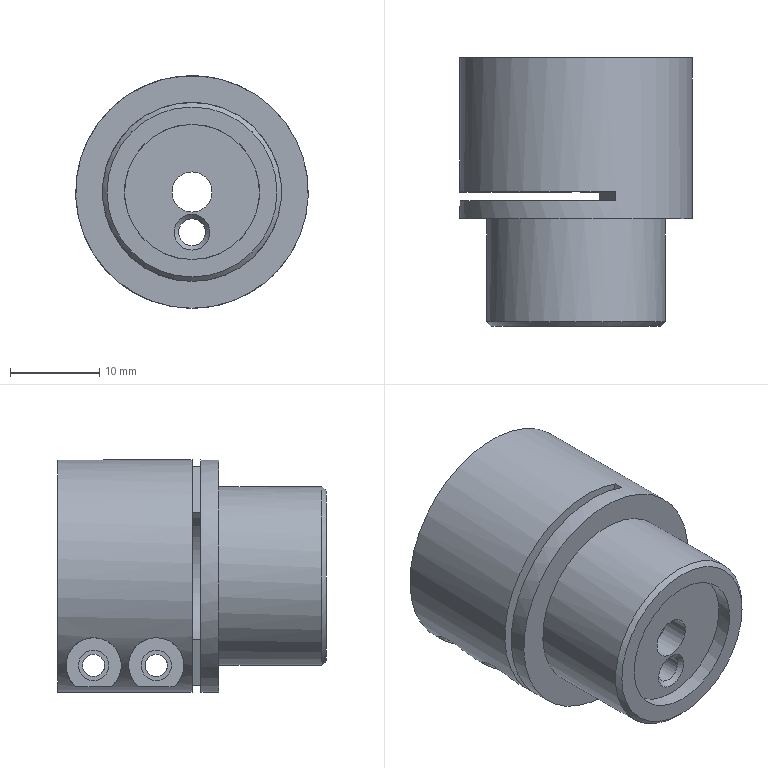Part | NX | 1 solid | 33 faces | box 26 x 30 x 26 mm | volume 7708 mm3 | plane 17 | cylinder 13 | cone 3 | commonest cylinder face diameters 15.1 x3 2.5 x2 3.4 x2 6.2 x2 3 x1 4.5 x1
STEP:
#1=CARTESIAN_POINT('',(0.,-15.,9.5));
#2=VERTEX_POINT('',#1);
#3=CARTESIAN_POINT('',(0.,-15.,0.));
#4=DIRECTION('',(0.,1.,0.));
#5=DIRECTION('',(0.,0.,1.));
#6=AXIS2_PLACEMENT_3D('',#3,#4,#5);
#7=CIRCLE('',#6,9.5);
#8=EDGE_CURVE('',#2,#2,#7,.F.);
#9=ORIENTED_EDGE('',*,*,#8,.T.);
#10=EDGE_LOOP('',(#9));
#11=FACE_BOUND('',#10,.T.);
#12=CARTESIAN_POINT('',(0.,-15.,7.55));
#13=VERTEX_POINT('',#12);
#14=CARTESIAN_POINT('',(0.,-15.,0.));
#15=DIRECTION('',(0.,1.,0.));
#16=DIRECTION('',(0.,0.,1.));
#17=AXIS2_PLACEMENT_3D('',#14,#15,#16);
#18=CIRCLE('',#17,7.55);
#19=EDGE_CURVE('',#13,#13,#18,.T.);
#20=ORIENTED_EDGE('',*,*,#19,.T.);
#21=EDGE_LOOP('',(#20));
#22=FACE_BOUND('',#21,.T.);
#23=CARTESIAN_POINT('',(0.,-15.,0.));
#24=DIRECTION('',(0.,1.,0.));
#25=DIRECTION('',(0.,0.,1.));
#26=AXIS2_PLACEMENT_3D('',#23,#24,#25);
#27=PLANE('',#26);
#28=ADVANCED_FACE('',(#11,#22),#27,.F.);
#29=CARTESIAN_POINT('',(4.446,-1.,12.216));
#30=VERTEX_POINT('',#29);
#31=CARTESIAN_POINT('',(4.446,0.,12.216));
#32=VERTEX_POINT('',#31);
#33=CARTESIAN_POINT('',(4.446,15.,12.216));
#34=DIRECTION('',(0.,-1.,0.));
#35=VECTOR('',#34,1000.);
#36=LINE('',#33,#35);
#37=EDGE_CURVE('',#30,#32,#36,.F.);
#38=ORIENTED_EDGE('',*,*,#37,.F.);
#39=CARTESIAN_POINT('',(4.446,-1.,-12.216));
#40=VERTEX_POINT('',#39);
#41=CARTESIAN_POINT('',(0.,-1.,0.));
#42=DIRECTION('',(0.,1.,0.));
#43=DIRECTION('',(0.,0.,1.));
#44=AXIS2_PLACEMENT_3D('',#41,#42,#43);
#45=CIRCLE('',#44,13.);
#46=EDGE_CURVE('',#40,#30,#45,.T.);
#47=ORIENTED_EDGE('',*,*,#46,.F.);
#48=CARTESIAN_POINT('',(4.446,0.,-12.216));
#49=VERTEX_POINT('',#48);
#50=CARTESIAN_POINT('',(4.446,15.,-12.216));
#51=DIRECTION('',(0.,-1.,0.));
#52=VECTOR('',#51,1000.);
#53=LINE('',#50,#52);
#54=EDGE_CURVE('',#40,#49,#53,.F.);
#55=ORIENTED_EDGE('',*,*,#54,.T.);
#56=CARTESIAN_POINT('',(0.5,0.,-12.99));
#57=VERTEX_POINT('',#56);
#58=CARTESIAN_POINT('',(0.,0.,0.));
#59=DIRECTION('',(0.,1.,0.));
#60=DIRECTION('',(0.,0.,1.));
#61=AXIS2_PLACEMENT_3D('',#58,#59,#60);
#62=CIRCLE('',#61,13.);
#63=EDGE_CURVE('',#49,#57,#62,.T.);
#64=ORIENTED_EDGE('',*,*,#63,.T.);
#65=CARTESIAN_POINT('',(0.5,15.,-12.99));
#66=VERTEX_POINT('',#65);
#67=CARTESIAN_POINT('',(0.5,15.,-12.99));
#68=DIRECTION('',(0.,-1.,0.));
#69=VECTOR('',#68,1000.);
#70=LINE('',#67,#69);
#71=EDGE_CURVE('',#57,#66,#70,.F.);
#72=ORIENTED_EDGE('',*,*,#71,.T.);
#73=CARTESIAN_POINT('',(-0.5,15.,-12.99));
#74=VERTEX_POINT('',#73);
#75=CARTESIAN_POINT('',(0.,15.,0.));
#76=DIRECTION('',(0.,1.,0.));
#77=DIRECTION('',(0.,0.,1.));
#78=AXIS2_PLACEMENT_3D('',#75,#76,#77);
#79=CIRCLE('',#78,13.);
#80=EDGE_CURVE('',#74,#66,#79,.T.);
#81=ORIENTED_EDGE('',*,*,#80,.F.);
#82=CARTESIAN_POINT('',(-0.5,0.,-12.99));
#83=VERTEX_POINT('',#82);
#84=CARTESIAN_POINT('',(-0.5,15.,-12.99));
#85=DIRECTION('',(0.,-1.,0.));
#86=VECTOR('',#85,1000.);
#87=LINE('',#84,#86);
#88=EDGE_CURVE('',#74,#83,#87,.T.);
#89=ORIENTED_EDGE('',*,*,#88,.T.);
#90=CARTESIAN_POINT('',(0.,0.,0.));
#91=DIRECTION('',(0.,1.,0.));
#92=DIRECTION('',(0.,0.,1.));
#93=AXIS2_PLACEMENT_3D('',#90,#91,#92);
#94=CIRCLE('',#93,13.);
#95=EDGE_CURVE('',#83,#32,#94,.T.);
#96=ORIENTED_EDGE('',*,*,#95,.T.);
#97=EDGE_LOOP('',(#38,#47,#55,#64,#72,#81,#89,#96));
#98=FACE_BOUND('',#97,.T.);
#99=CARTESIAN_POINT('',(-4.,5.999,-12.369));
#100=VERTEX_POINT('',#99);
#101=CARTESIAN_POINT('',(-4.,2.001,-12.369));
#102=VERTEX_POINT('',#101);
#103=CARTESIAN_POINT('',(-4.,5.999,-12.369));
#104=CARTESIAN_POINT('',(-4.809,6.309,-12.108));
#105=CARTESIAN_POINT('',(-6.367,6.865,-11.433));
#106=CARTESIAN_POINT('',(-8.603,7.27,-9.884));
#107=CARTESIAN_POINT('',(-10.159,6.725,-8.173));
#108=CARTESIAN_POINT('',(-10.887,5.376,-7.115));
#109=CARTESIAN_POINT('',(-11.081,4.013,-6.796));
#110=CARTESIAN_POINT('',(-10.895,2.65,-7.102));
#111=CARTESIAN_POINT('',(-10.168,1.277,-8.163));
#112=CARTESIAN_POINT('',(-8.611,0.7311,-9.877));
#113=CARTESIAN_POINT('',(-6.379,1.131,-11.427));
#114=CARTESIAN_POINT('',(-4.811,1.69,-12.107));
#115=CARTESIAN_POINT('',(-4.,2.001,-12.369));
#116=B_SPLINE_CURVE_WITH_KNOTS('',3,(#103,#104,#105,#106,#107,#108,#109,#110,#111,#112,#113,#114,#115),.UNSPECIFIED.,.F.,.F.,(4,1,1,1,1,1,1,1,1,1,4),(0.,0.00268,0.00536,0.008039,0.009379,0.01072,0.01206,0.0134,0.01608,0.01876,0.02144),.UNSPECIFIED.);
#117=EDGE_CURVE('',#100,#102,#116,.T.);
#118=ORIENTED_EDGE('',*,*,#117,.T.);
#119=CARTESIAN_POINT('',(-4.,15.,-12.369));
#120=DIRECTION('',(0.,-1.,0.));
#121=VECTOR('',#120,1000.);
#122=LINE('',#119,#121);
#123=EDGE_CURVE('',#102,#100,#122,.F.);
#124=ORIENTED_EDGE('',*,*,#123,.T.);
#125=EDGE_LOOP('',(#118,#124));
#126=FACE_BOUND('',#125,.T.);
#127=CARTESIAN_POINT('',(-4.,12.999,-12.369));
#128=VERTEX_POINT('',#127);
#129=CARTESIAN_POINT('',(-4.,9.001,-12.369));
#130=VERTEX_POINT('',#129);
#131=CARTESIAN_POINT('',(-4.,12.999,-12.369));
#132=CARTESIAN_POINT('',(-4.809,13.309,-12.108));
#133=CARTESIAN_POINT('',(-6.367,13.865,-11.433));
#134=CARTESIAN_POINT('',(-8.603,14.27,-9.884));
#135=CARTESIAN_POINT('',(-10.159,13.725,-8.173));
#136=CARTESIAN_POINT('',(-10.887,12.376,-7.115));
#137=CARTESIAN_POINT('',(-11.081,11.013,-6.796));
#138=CARTESIAN_POINT('',(-10.895,9.65,-7.102));
#139=CARTESIAN_POINT('',(-10.168,8.277,-8.163));
#140=CARTESIAN_POINT('',(-8.611,7.731,-9.877));
#141=CARTESIAN_POINT('',(-6.379,8.131,-11.427));
#142=CARTESIAN_POINT('',(-4.811,8.69,-12.107));
#143=CARTESIAN_POINT('',(-4.,9.001,-12.369));
#144=B_SPLINE_CURVE_WITH_KNOTS('',3,(#131,#132,#133,#134,#135,#136,#137,#138,#139,#140,#141,#142,#143),.UNSPECIFIED.,.F.,.F.,(4,1,1,1,1,1,1,1,1,1,4),(0.,0.00268,0.00536,0.008039,0.009379,0.01072,0.01206,0.0134,0.01608,0.01876,0.02144),.UNSPECIFIED.);
#145=EDGE_CURVE('',#128,#130,#144,.T.);
#146=ORIENTED_EDGE('',*,*,#145,.T.);
#147=CARTESIAN_POINT('',(-4.,15.,-12.369));
#148=DIRECTION('',(0.,-1.,0.));
#149=VECTOR('',#148,1000.);
#150=LINE('',#147,#149);
#151=EDGE_CURVE('',#130,#128,#150,.F.);
#152=ORIENTED_EDGE('',*,*,#151,.T.);
#153=EDGE_LOOP('',(#146,#152));
#154=FACE_BOUND('',#153,.T.);
#155=CARTESIAN_POINT('',(9.614,4.,-8.75));
#156=VERTEX_POINT('',#155);
#157=CARTESIAN_POINT('',(9.506,3.358,-8.871));
#158=CARTESIAN_POINT('',(9.669,4.,-8.69));
#159=CARTESIAN_POINT('',(9.506,4.642,-8.871));
#160=CARTESIAN_POINT('',(9.013,5.175,-9.383));
#161=CARTESIAN_POINT('',(8.2,5.33,-10.117));
#162=CARTESIAN_POINT('',(7.34,5.068,-10.742));
#163=CARTESIAN_POINT('',(6.716,4.613,-11.134));
#164=CARTESIAN_POINT('',(6.411,3.991,-11.309));
#165=CARTESIAN_POINT('',(6.726,3.378,-11.128));
#166=CARTESIAN_POINT('',(7.348,2.929,-10.736));
#167=CARTESIAN_POINT('',(8.201,2.671,-10.116));
#168=CARTESIAN_POINT('',(9.016,2.826,-9.38));
#169=CARTESIAN_POINT('',(9.506,3.358,-8.871));
#170=CARTESIAN_POINT('',(9.669,4.,-8.69));
#171=CARTESIAN_POINT('',(9.506,4.642,-8.871));
#172=B_SPLINE_CURVE_WITH_KNOTS('',3,(#157,#158,#159,#160,#161,#162,#163,#164,#165,#166,#167,#168,#169,#170,#171),.UNSPECIFIED.,.T.,.F.,(1,1,1,1,1,1,1,1,1,1,1,1,1,1,1,1,1,1,1),(-0.002581,-0.001291,-0.0006453,0.,0.0006453,0.001291,0.002581,0.003872,0.004517,0.005162,0.005808,0.006453,0.007744,0.009034,0.00968,0.01032,0.01097,0.01162,0.01291),.UNSPECIFIED.);
#173=EDGE_CURVE('',#156,#156,#172,.T.);
#174=ORIENTED_EDGE('',*,*,#173,.T.);
#175=EDGE_LOOP('',(#174));
#176=FACE_BOUND('',#175,.T.);
#177=CARTESIAN_POINT('',(9.614,11.,-8.75));
#178=VERTEX_POINT('',#177);
#179=CARTESIAN_POINT('',(9.506,10.358,-8.871));
#180=CARTESIAN_POINT('',(9.669,11.,-8.69));
#181=CARTESIAN_POINT('',(9.506,11.642,-8.871));
#182=CARTESIAN_POINT('',(9.013,12.175,-9.383));
#183=CARTESIAN_POINT('',(8.2,12.33,-10.117));
#184=CARTESIAN_POINT('',(7.34,12.068,-10.742));
#185=CARTESIAN_POINT('',(6.716,11.613,-11.134));
#186=CARTESIAN_POINT('',(6.411,10.991,-11.309));
#187=CARTESIAN_POINT('',(6.726,10.378,-11.128));
#188=CARTESIAN_POINT('',(7.348,9.929,-10.736));
#189=CARTESIAN_POINT('',(8.201,9.671,-10.116));
#190=CARTESIAN_POINT('',(9.016,9.826,-9.38));
#191=CARTESIAN_POINT('',(9.506,10.358,-8.871));
#192=CARTESIAN_POINT('',(9.669,11.,-8.69));
#193=CARTESIAN_POINT('',(9.506,11.642,-8.871));
#194=B_SPLINE_CURVE_WITH_KNOTS('',3,(#179,#180,#181,#182,#183,#184,#185,#186,#187,#188,#189,#190,#191,#192,#193),.UNSPECIFIED.,.T.,.F.,(1,1,1,1,1,1,1,1,1,1,1,1,1,1,1,1,1,1,1),(-0.002581,-0.001291,-0.0006453,0.,0.0006453,0.001291,0.002581,0.003872,0.004517,0.005162,0.005808,0.006453,0.007744,0.009034,0.00968,0.01032,0.01097,0.01162,0.01291),.UNSPECIFIED.);
#195=EDGE_CURVE('',#178,#178,#194,.T.);
#196=ORIENTED_EDGE('',*,*,#195,.T.);
#197=EDGE_LOOP('',(#196));
#198=FACE_BOUND('',#197,.T.);
#199=CARTESIAN_POINT('',(0.,-3.,-13.));
#200=VERTEX_POINT('',#199);
#201=CARTESIAN_POINT('',(0.,-3.,0.));
#202=DIRECTION('',(0.,-1.,0.));
#203=DIRECTION('',(0.,0.,-1.));
#204=AXIS2_PLACEMENT_3D('',#201,#202,#203);
#205=CIRCLE('',#204,13.);
#206=EDGE_CURVE('',#200,#200,#205,.T.);
#207=ORIENTED_EDGE('',*,*,#206,.F.);
#208=EDGE_LOOP('',(#207));
#209=FACE_BOUND('',#208,.T.);
#210=CARTESIAN_POINT('',(0.,15.,0.));
#211=DIRECTION('',(0.,-1.,0.));
#212=DIRECTION('',(0.,0.,-1.));
#213=AXIS2_PLACEMENT_3D('',#210,#211,#212);
#214=CYLINDRICAL_SURFACE('',#213,13.);
#215=ADVANCED_FACE('',(#98,#126,#154,#176,#198,#209),#214,.T.);
#216=CARTESIAN_POINT('',(2.582,-1.,-7.095));
#217=VERTEX_POINT('',#216);
#218=CARTESIAN_POINT('',(2.582,0.,-7.095));
#219=VERTEX_POINT('',#218);
#220=CARTESIAN_POINT('',(2.582,15.,-7.095));
#221=DIRECTION('',(0.,-1.,0.));
#222=VECTOR('',#221,1000.);
#223=LINE('',#220,#222);
#224=EDGE_CURVE('',#217,#219,#223,.F.);
#225=ORIENTED_EDGE('',*,*,#224,.F.);
#226=CARTESIAN_POINT('',(2.582,-1.,7.095));
#227=VERTEX_POINT('',#226);
#228=CARTESIAN_POINT('',(0.,-1.,0.));
#229=DIRECTION('',(0.,1.,0.));
#230=DIRECTION('',(0.,0.,1.));
#231=AXIS2_PLACEMENT_3D('',#228,#229,#230);
#232=CIRCLE('',#231,7.55);
#233=EDGE_CURVE('',#217,#227,#232,.T.);
#234=ORIENTED_EDGE('',*,*,#233,.T.);
#235=CARTESIAN_POINT('',(2.582,0.,7.095));
#236=VERTEX_POINT('',#235);
#237=CARTESIAN_POINT('',(2.582,15.,7.095));
#238=DIRECTION('',(0.,-1.,0.));
#239=VECTOR('',#238,1000.);
#240=LINE('',#237,#239);
#241=EDGE_CURVE('',#227,#236,#240,.F.);
#242=ORIENTED_EDGE('',*,*,#241,.T.);
#243=CARTESIAN_POINT('',(0.5,0.,7.533));
#244=VERTEX_POINT('',#243);
#245=CARTESIAN_POINT('',(0.,0.,0.));
#246=DIRECTION('',(0.,1.,0.));
#247=DIRECTION('',(0.,0.,1.));
#248=AXIS2_PLACEMENT_3D('',#245,#246,#247);
#249=CIRCLE('',#248,7.55);
#250=EDGE_CURVE('',#244,#236,#249,.T.);
#251=ORIENTED_EDGE('',*,*,#250,.F.);
#252=CARTESIAN_POINT('',(0.5,15.,7.533));
#253=VERTEX_POINT('',#252);
#254=CARTESIAN_POINT('',(0.5,15.,7.533));
#255=DIRECTION('',(0.,-1.,0.));
#256=VECTOR('',#255,1000.);
#257=LINE('',#254,#256);
#258=EDGE_CURVE('',#253,#244,#257,.T.);
#259=ORIENTED_EDGE('',*,*,#258,.F.);
#260=CARTESIAN_POINT('',(0.5,15.,-7.533));
#261=VERTEX_POINT('',#260);
#262=CARTESIAN_POINT('',(0.,15.,0.));
#263=DIRECTION('',(0.,1.,0.));
#264=DIRECTION('',(0.,0.,1.));
#265=AXIS2_PLACEMENT_3D('',#262,#263,#264);
#266=CIRCLE('',#265,7.55);
#267=EDGE_CURVE('',#253,#261,#266,.T.);
#268=ORIENTED_EDGE('',*,*,#267,.T.);
#269=CARTESIAN_POINT('',(0.5,0.,-7.533));
#270=VERTEX_POINT('',#269);
#271=CARTESIAN_POINT('',(0.5,15.,-7.533));
#272=DIRECTION('',(0.,-1.,0.));
#273=VECTOR('',#272,1000.);
#274=LINE('',#271,#273);
#275=EDGE_CURVE('',#270,#261,#274,.F.);
#276=ORIENTED_EDGE('',*,*,#275,.F.);
#277=CARTESIAN_POINT('',(0.,0.,0.));
#278=DIRECTION('',(0.,1.,0.));
#279=DIRECTION('',(0.,0.,1.));
#280=AXIS2_PLACEMENT_3D('',#277,#278,#279);
#281=CIRCLE('',#280,7.55);
#282=EDGE_CURVE('',#219,#270,#281,.T.);
#283=ORIENTED_EDGE('',*,*,#282,.F.);
#284=EDGE_LOOP('',(#225,#234,#242,#251,#259,#268,#276,#283));
#285=FACE_BOUND('',#284,.T.);
#286=CARTESIAN_POINT('',(0.,-10.3,-7.55));
#287=VERTEX_POINT('',#286);
#288=CARTESIAN_POINT('',(0.,-10.3,0.));
#289=DIRECTION('',(0.,-1.,0.));
#290=DIRECTION('',(0.,0.,-1.));
#291=AXIS2_PLACEMENT_3D('',#288,#289,#290);
#292=CIRCLE('',#291,7.55);
#293=EDGE_CURVE('',#287,#287,#292,.T.);
#294=ORIENTED_EDGE('',*,*,#293,.T.);
#295=EDGE_LOOP('',(#294));
#296=FACE_BOUND('',#295,.T.);
#297=CARTESIAN_POINT('',(0.,15.,0.));
#298=DIRECTION('',(0.,-1.,0.));
#299=DIRECTION('',(0.,0.,-1.));
#300=AXIS2_PLACEMENT_3D('',#297,#298,#299);
#301=CYLINDRICAL_SURFACE('',#300,7.55);
#302=ADVANCED_FACE('',(#285,#296),#301,.F.);
#303=CARTESIAN_POINT('',(0.,-13.3,-7.55));
#304=VERTEX_POINT('',#303);
#305=CARTESIAN_POINT('',(0.,-13.3,0.));
#306=DIRECTION('',(0.,-1.,0.));
#307=DIRECTION('',(0.,0.,-1.));
#308=AXIS2_PLACEMENT_3D('',#305,#306,#307);
#309=CIRCLE('',#308,7.55);
#310=EDGE_CURVE('',#304,#304,#309,.T.);
#311=ORIENTED_EDGE('',*,*,#310,.F.);
#312=EDGE_LOOP('',(#311));
#313=FACE_BOUND('',#312,.T.);
#314=ORIENTED_EDGE('',*,*,#19,.F.);
#315=EDGE_LOOP('',(#314));
#316=FACE_BOUND('',#315,.T.);
#317=CARTESIAN_POINT('',(0.,15.,0.));
#318=DIRECTION('',(0.,-1.,0.));
#319=DIRECTION('',(0.,0.,-1.));
#320=AXIS2_PLACEMENT_3D('',#317,#318,#319);
#321=CYLINDRICAL_SURFACE('',#320,7.55);
#322=ADVANCED_FACE('',(#313,#316),#321,.F.);
#323=CARTESIAN_POINT('',(-0.5,15.,-7.533));
#324=VERTEX_POINT('',#323);
#325=CARTESIAN_POINT('',(-0.5,15.,9.55));
#326=DIRECTION('',(0.,0.,1.));
#327=VECTOR('',#326,1000.);
#328=LINE('',#325,#327);
#329=EDGE_CURVE('',#74,#324,#328,.T.);
#330=ORIENTED_EDGE('',*,*,#329,.F.);
#331=ORIENTED_EDGE('',*,*,#80,.T.);
#332=CARTESIAN_POINT('',(0.5,15.,9.55));
#333=DIRECTION('',(0.,0.,-1.));
#334=VECTOR('',#333,1000.);
#335=LINE('',#332,#334);
#336=EDGE_CURVE('',#261,#66,#335,.T.);
#337=ORIENTED_EDGE('',*,*,#336,.F.);
#338=ORIENTED_EDGE('',*,*,#267,.F.);
#339=CARTESIAN_POINT('',(0.5,15.,9.55));
#340=VERTEX_POINT('',#339);
#341=CARTESIAN_POINT('',(0.5,15.,9.55));
#342=DIRECTION('',(0.,0.,-1.));
#343=VECTOR('',#342,1000.);
#344=LINE('',#341,#343);
#345=EDGE_CURVE('',#340,#253,#344,.T.);
#346=ORIENTED_EDGE('',*,*,#345,.F.);
#347=CARTESIAN_POINT('',(-0.5,15.,9.55));
#348=VERTEX_POINT('',#347);
#349=CARTESIAN_POINT('',(0.5,15.,9.55));
#350=DIRECTION('',(1.,0.,0.));
#351=VECTOR('',#350,1000.);
#352=LINE('',#349,#351);
#353=EDGE_CURVE('',#348,#340,#352,.T.);
#354=ORIENTED_EDGE('',*,*,#353,.F.);
#355=CARTESIAN_POINT('',(-0.5,15.,7.533));
#356=VERTEX_POINT('',#355);
#357=CARTESIAN_POINT('',(-0.5,15.,9.55));
#358=DIRECTION('',(0.,0.,1.));
#359=VECTOR('',#358,1000.);
#360=LINE('',#357,#359);
#361=EDGE_CURVE('',#356,#348,#360,.T.);
#362=ORIENTED_EDGE('',*,*,#361,.F.);
#363=CARTESIAN_POINT('',(0.,15.,0.));
#364=DIRECTION('',(0.,1.,0.));
#365=DIRECTION('',(0.,0.,1.));
#366=AXIS2_PLACEMENT_3D('',#363,#364,#365);
#367=CIRCLE('',#366,7.55);
#368=EDGE_CURVE('',#324,#356,#367,.T.);
#369=ORIENTED_EDGE('',*,*,#368,.F.);
#370=EDGE_LOOP('',(#330,#331,#337,#338,#346,#354,#362,#369));
#371=FACE_BOUND('',#370,.T.);
#372=CARTESIAN_POINT('',(0.,15.,0.));
#373=DIRECTION('',(0.,1.,0.));
#374=DIRECTION('',(0.,0.,1.));
#375=AXIS2_PLACEMENT_3D('',#372,#373,#374);
#376=PLANE('',#375);
#377=ADVANCED_FACE('',(#371),#376,.T.);
#378=CARTESIAN_POINT('',(-0.5,0.,-7.533));
#379=VERTEX_POINT('',#378);
#380=CARTESIAN_POINT('',(-0.5,0.,7.533));
#381=VERTEX_POINT('',#380);
#382=CARTESIAN_POINT('',(0.,0.,0.));
#383=DIRECTION('',(0.,1.,0.));
#384=DIRECTION('',(0.,0.,1.));
#385=AXIS2_PLACEMENT_3D('',#382,#383,#384);
#386=CIRCLE('',#385,7.55);
#387=EDGE_CURVE('',#379,#381,#386,.T.);
#388=ORIENTED_EDGE('',*,*,#387,.F.);
#389=CARTESIAN_POINT('',(-0.5,15.,-7.533));
#390=DIRECTION('',(0.,-1.,0.));
#391=VECTOR('',#390,1000.);
#392=LINE('',#389,#391);
#393=EDGE_CURVE('',#324,#379,#392,.T.);
#394=ORIENTED_EDGE('',*,*,#393,.F.);
#395=ORIENTED_EDGE('',*,*,#368,.T.);
#396=CARTESIAN_POINT('',(-0.5,15.,7.533));
#397=DIRECTION('',(0.,-1.,0.));
#398=VECTOR('',#397,1000.);
#399=LINE('',#396,#398);
#400=EDGE_CURVE('',#381,#356,#399,.F.);
#401=ORIENTED_EDGE('',*,*,#400,.F.);
#402=EDGE_LOOP('',(#388,#394,#395,#401));
#403=FACE_BOUND('',#402,.T.);
#404=CARTESIAN_POINT('',(0.,15.,0.));
#405=DIRECTION('',(0.,-1.,0.));
#406=DIRECTION('',(0.,0.,-1.));
#407=AXIS2_PLACEMENT_3D('',#404,#405,#406);
#408=CYLINDRICAL_SURFACE('',#407,7.55);
#409=ADVANCED_FACE('',(#403),#408,.F.);
#410=ORIENTED_EDGE('',*,*,#258,.T.);
#411=CARTESIAN_POINT('',(0.5,0.,9.55));
#412=VERTEX_POINT('',#411);
#413=CARTESIAN_POINT('',(0.5,0.,9.55));
#414=DIRECTION('',(0.,0.,1.));
#415=VECTOR('',#414,1000.);
#416=LINE('',#413,#415);
#417=EDGE_CURVE('',#244,#412,#416,.T.);
#418=ORIENTED_EDGE('',*,*,#417,.T.);
#419=CARTESIAN_POINT('',(0.5,-1.,9.55));
#420=DIRECTION('',(0.,1.,0.));
#421=VECTOR('',#420,1000.);
#422=LINE('',#419,#421);
#423=EDGE_CURVE('',#412,#340,#422,.T.);
#424=ORIENTED_EDGE('',*,*,#423,.T.);
#425=ORIENTED_EDGE('',*,*,#345,.T.);
#426=EDGE_LOOP('',(#410,#418,#424,#425));
#427=FACE_BOUND('',#426,.T.);
#428=CARTESIAN_POINT('',(0.5,-1.,9.55));
#429=DIRECTION('',(1.,0.,0.));
#430=DIRECTION('',(0.,0.,-1.));
#431=AXIS2_PLACEMENT_3D('',#428,#429,#430);
#432=PLANE('',#431);
#433=ADVANCED_FACE('',(#427),#432,.F.);
#434=CARTESIAN_POINT('',(-0.5,0.,9.55));
#435=VERTEX_POINT('',#434);
#436=CARTESIAN_POINT('',(-0.5,-1.,9.55));
#437=DIRECTION('',(0.,1.,0.));
#438=VECTOR('',#437,1000.);
#439=LINE('',#436,#438);
#440=EDGE_CURVE('',#435,#348,#439,.T.);
#441=ORIENTED_EDGE('',*,*,#440,.F.);
#442=CARTESIAN_POINT('',(-0.5,0.,9.55));
#443=DIRECTION('',(0.,0.,-1.));
#444=VECTOR('',#443,1000.);
#445=LINE('',#442,#444);
#446=EDGE_CURVE('',#435,#381,#445,.T.);
#447=ORIENTED_EDGE('',*,*,#446,.T.);
#448=ORIENTED_EDGE('',*,*,#400,.T.);
#449=ORIENTED_EDGE('',*,*,#361,.T.);
#450=EDGE_LOOP('',(#441,#447,#448,#449));
#451=FACE_BOUND('',#450,.T.);
#452=CARTESIAN_POINT('',(-0.5,-1.,9.55));
#453=DIRECTION('',(-1.,0.,0.));
#454=DIRECTION('',(0.,0.,1.));
#455=AXIS2_PLACEMENT_3D('',#452,#453,#454);
#456=PLANE('',#455);
#457=ADVANCED_FACE('',(#451),#456,.F.);
#458=ORIENTED_EDGE('',*,*,#423,.F.);
#459=CARTESIAN_POINT('',(0.5,0.,9.55));
#460=DIRECTION('',(-1.,0.,0.));
#461=VECTOR('',#460,1000.);
#462=LINE('',#459,#461);
#463=EDGE_CURVE('',#412,#435,#462,.T.);
#464=ORIENTED_EDGE('',*,*,#463,.T.);
#465=ORIENTED_EDGE('',*,*,#440,.T.);
#466=ORIENTED_EDGE('',*,*,#353,.T.);
#467=EDGE_LOOP('',(#458,#464,#465,#466));
#468=FACE_BOUND('',#467,.T.);
#469=CARTESIAN_POINT('',(0.5,-1.,9.55));
#470=DIRECTION('',(0.,0.,1.));
#471=DIRECTION('',(1.,0.,0.));
#472=AXIS2_PLACEMENT_3D('',#469,#470,#471);
#473=PLANE('',#472);
#474=ADVANCED_FACE('',(#468),#473,.F.);
#475=CARTESIAN_POINT('',(-0.5,11.,-8.3));
#476=VERTEX_POINT('',#475);
#477=CARTESIAN_POINT('',(-0.5,11.,-10.));
#478=DIRECTION('',(-1.,0.,0.));
#479=DIRECTION('',(0.,0.,1.));
#480=AXIS2_PLACEMENT_3D('',#477,#478,#479);
#481=CIRCLE('',#480,1.7);
#482=EDGE_CURVE('',#476,#476,#481,.T.);
#483=ORIENTED_EDGE('',*,*,#482,.T.);
#484=EDGE_LOOP('',(#483));
#485=FACE_BOUND('',#484,.T.);
#486=CARTESIAN_POINT('',(-0.5,4.,-8.3));
#487=VERTEX_POINT('',#486);
#488=CARTESIAN_POINT('',(-0.5,4.,-10.));
#489=DIRECTION('',(-1.,0.,0.));
#490=DIRECTION('',(0.,0.,1.));
#491=AXIS2_PLACEMENT_3D('',#488,#489,#490);
#492=CIRCLE('',#491,1.7);
#493=EDGE_CURVE('',#487,#487,#492,.T.);
#494=ORIENTED_EDGE('',*,*,#493,.T.);
#495=EDGE_LOOP('',(#494));
#496=FACE_BOUND('',#495,.T.);
#497=ORIENTED_EDGE('',*,*,#393,.T.);
#498=CARTESIAN_POINT('',(-0.5,0.,9.55));
#499=DIRECTION('',(0.,0.,-1.));
#500=VECTOR('',#499,1000.);
#501=LINE('',#498,#500);
#502=EDGE_CURVE('',#379,#83,#501,.T.);
#503=ORIENTED_EDGE('',*,*,#502,.T.);
#504=ORIENTED_EDGE('',*,*,#88,.F.);
#505=ORIENTED_EDGE('',*,*,#329,.T.);
#506=EDGE_LOOP('',(#497,#503,#504,#505));
#507=FACE_BOUND('',#506,.T.);
#508=CARTESIAN_POINT('',(-0.5,-1.,9.55));
#509=DIRECTION('',(-1.,0.,0.));
#510=DIRECTION('',(0.,0.,1.));
#511=AXIS2_PLACEMENT_3D('',#508,#509,#510);
#512=PLANE('',#511);
#513=ADVANCED_FACE('',(#485,#496,#507),#512,.F.);
#514=CARTESIAN_POINT('',(0.5,11.,-8.75));
#515=VERTEX_POINT('',#514);
#516=CARTESIAN_POINT('',(0.5,11.,-10.));
#517=DIRECTION('',(-1.,0.,0.));
#518=DIRECTION('',(0.,0.,1.));
#519=AXIS2_PLACEMENT_3D('',#516,#517,#518);
#520=CIRCLE('',#519,1.25);
#521=EDGE_CURVE('',#515,#515,#520,.T.);
#522=ORIENTED_EDGE('',*,*,#521,.F.);
#523=EDGE_LOOP('',(#522));
#524=FACE_BOUND('',#523,.T.);
#525=CARTESIAN_POINT('',(0.5,4.,-8.75));
#526=VERTEX_POINT('',#525);
#527=CARTESIAN_POINT('',(0.5,4.,-10.));
#528=DIRECTION('',(-1.,0.,0.));
#529=DIRECTION('',(0.,0.,1.));
#530=AXIS2_PLACEMENT_3D('',#527,#528,#529);
#531=CIRCLE('',#530,1.25);
#532=EDGE_CURVE('',#526,#526,#531,.T.);
#533=ORIENTED_EDGE('',*,*,#532,.F.);
#534=EDGE_LOOP('',(#533));
#535=FACE_BOUND('',#534,.T.);
#536=ORIENTED_EDGE('',*,*,#71,.F.);
#537=CARTESIAN_POINT('',(0.5,0.,9.55));
#538=DIRECTION('',(0.,0.,1.));
#539=VECTOR('',#538,1000.);
#540=LINE('',#537,#539);
#541=EDGE_CURVE('',#57,#270,#540,.T.);
#542=ORIENTED_EDGE('',*,*,#541,.T.);
#543=ORIENTED_EDGE('',*,*,#275,.T.);
#544=ORIENTED_EDGE('',*,*,#336,.T.);
#545=EDGE_LOOP('',(#536,#542,#543,#544));
#546=FACE_BOUND('',#545,.T.);
#547=CARTESIAN_POINT('',(0.5,-1.,9.55));
#548=DIRECTION('',(1.,0.,0.));
#549=DIRECTION('',(0.,0.,-1.));
#550=AXIS2_PLACEMENT_3D('',#547,#548,#549);
#551=PLANE('',#550);
#552=ADVANCED_FACE('',(#524,#535,#546),#551,.F.);
#553=CARTESIAN_POINT('',(0.,-1.,0.));
#554=DIRECTION('',(0.342,0.,0.9397));
#555=VECTOR('',#554,1000.);
#556=LINE('',#553,#555);
#557=EDGE_CURVE('',#227,#30,#556,.T.);
#558=ORIENTED_EDGE('',*,*,#557,.F.);
#559=ORIENTED_EDGE('',*,*,#233,.F.);
#560=CARTESIAN_POINT('',(0.,-1.,0.));
#561=DIRECTION('',(0.342,0.,-0.9397));
#562=VECTOR('',#561,1000.);
#563=LINE('',#560,#562);
#564=EDGE_CURVE('',#217,#40,#563,.T.);
#565=ORIENTED_EDGE('',*,*,#564,.T.);
#566=ORIENTED_EDGE('',*,*,#46,.T.);
#567=EDGE_LOOP('',(#558,#559,#565,#566));
#568=FACE_BOUND('',#567,.T.);
#569=CARTESIAN_POINT('',(0.,-1.,0.));
#570=DIRECTION('',(0.,1.,0.));
#571=DIRECTION('',(0.,0.,1.));
#572=AXIS2_PLACEMENT_3D('',#569,#570,#571);
#573=PLANE('',#572);
#574=ADVANCED_FACE('',(#568),#573,.T.);
#575=CARTESIAN_POINT('',(5.13,0.,-14.095));
#576=DIRECTION('',(-0.342,0.,0.9397));
#577=VECTOR('',#576,1000.);
#578=LINE('',#575,#577);
#579=EDGE_CURVE('',#49,#219,#578,.T.);
#580=ORIENTED_EDGE('',*,*,#579,.T.);
#581=ORIENTED_EDGE('',*,*,#282,.T.);
#582=ORIENTED_EDGE('',*,*,#541,.F.);
#583=ORIENTED_EDGE('',*,*,#63,.F.);
#584=EDGE_LOOP('',(#580,#581,#582,#583));
#585=FACE_BOUND('',#584,.T.);
#586=CARTESIAN_POINT('',(5.13,0.,14.095));
#587=DIRECTION('',(0.,1.,0.));
#588=DIRECTION('',(0.,0.,1.));
#589=AXIS2_PLACEMENT_3D('',#586,#587,#588);
#590=PLANE('',#589);
#591=ADVANCED_FACE('',(#585),#590,.F.);
#592=ORIENTED_EDGE('',*,*,#564,.F.);
#593=ORIENTED_EDGE('',*,*,#224,.T.);
#594=ORIENTED_EDGE('',*,*,#579,.F.);
#595=ORIENTED_EDGE('',*,*,#54,.F.);
#596=EDGE_LOOP('',(#592,#593,#594,#595));
#597=FACE_BOUND('',#596,.T.);
#598=CARTESIAN_POINT('',(0.,0.,0.));
#599=DIRECTION('',(0.9397,0.,0.342));
#600=DIRECTION('',(0.342,0.,-0.9397));
#601=AXIS2_PLACEMENT_3D('',#598,#599,#600);
#602=PLANE('',#601);
#603=ADVANCED_FACE('',(#597),#602,.F.);
#604=ORIENTED_EDGE('',*,*,#37,.T.);
#605=CARTESIAN_POINT('',(5.13,0.,14.095));
#606=DIRECTION('',(-0.342,0.,-0.9397));
#607=VECTOR('',#606,1000.);
#608=LINE('',#605,#607);
#609=EDGE_CURVE('',#32,#236,#608,.T.);
#610=ORIENTED_EDGE('',*,*,#609,.T.);
#611=ORIENTED_EDGE('',*,*,#241,.F.);
#612=ORIENTED_EDGE('',*,*,#557,.T.);
#613=EDGE_LOOP('',(#604,#610,#611,#612));
#614=FACE_BOUND('',#613,.T.);
#615=CARTESIAN_POINT('',(0.,0.,0.));
#616=DIRECTION('',(-0.9397,0.,0.342));
#617=DIRECTION('',(0.342,0.,0.9397));
#618=AXIS2_PLACEMENT_3D('',#615,#616,#617);
#619=PLANE('',#618);
#620=ADVANCED_FACE('',(#614),#619,.T.);
#621=ORIENTED_EDGE('',*,*,#250,.T.);
#622=ORIENTED_EDGE('',*,*,#609,.F.);
#623=ORIENTED_EDGE('',*,*,#95,.F.);
#624=ORIENTED_EDGE('',*,*,#502,.F.);
#625=ORIENTED_EDGE('',*,*,#387,.T.);
#626=ORIENTED_EDGE('',*,*,#446,.F.);
#627=ORIENTED_EDGE('',*,*,#463,.F.);
#628=ORIENTED_EDGE('',*,*,#417,.F.);
#629=EDGE_LOOP('',(#621,#622,#623,#624,#625,#626,#627,#628));
#630=FACE_BOUND('',#629,.T.);
#631=CARTESIAN_POINT('',(5.13,0.,14.095));
#632=DIRECTION('',(0.,1.,0.));
#633=DIRECTION('',(0.,0.,1.));
#634=AXIS2_PLACEMENT_3D('',#631,#632,#633);
#635=PLANE('',#634);
#636=ADVANCED_FACE('',(#630),#635,.F.);
#637=CARTESIAN_POINT('',(-4.,4.,-8.3));
#638=VERTEX_POINT('',#637);
#639=CARTESIAN_POINT('',(-4.,4.,-10.));
#640=DIRECTION('',(-1.,0.,0.));
#641=DIRECTION('',(0.,0.,1.));
#642=AXIS2_PLACEMENT_3D('',#639,#640,#641);
#643=CIRCLE('',#642,1.7);
#644=EDGE_CURVE('',#638,#638,#643,.T.);
#645=ORIENTED_EDGE('',*,*,#644,.F.);
#646=EDGE_LOOP('',(#645));
#647=FACE_BOUND('',#646,.T.);
#648=CARTESIAN_POINT('',(-4.,4.,-10.));
#649=DIRECTION('',(-1.,0.,0.));
#650=DIRECTION('',(0.,0.,1.));
#651=AXIS2_PLACEMENT_3D('',#648,#649,#650);
#652=CIRCLE('',#651,3.1);
#653=EDGE_CURVE('',#102,#100,#652,.T.);
#654=ORIENTED_EDGE('',*,*,#653,.T.);
#655=ORIENTED_EDGE('',*,*,#123,.F.);
#656=EDGE_LOOP('',(#654,#655));
#657=FACE_BOUND('',#656,.T.);
#658=CARTESIAN_POINT('',(-4.,5.7,-10.));
#659=DIRECTION('',(1.,0.,0.));
#660=DIRECTION('',(0.,0.,-1.));
#661=AXIS2_PLACEMENT_3D('',#658,#659,#660);
#662=PLANE('',#661);
#663=ADVANCED_FACE('',(#647,#657),#662,.F.);
#664=ORIENTED_EDGE('',*,*,#653,.F.);
#665=ORIENTED_EDGE('',*,*,#117,.F.);
#666=EDGE_LOOP('',(#664,#665));
#667=FACE_BOUND('',#666,.T.);
#668=CARTESIAN_POINT('',(-15.,4.,-10.));
#669=DIRECTION('',(-1.,0.,0.));
#670=DIRECTION('',(0.,0.,1.));
#671=AXIS2_PLACEMENT_3D('',#668,#669,#670);
#672=CYLINDRICAL_SURFACE('',#671,3.1);
#673=ADVANCED_FACE('',(#667),#672,.F.);
#674=ORIENTED_EDGE('',*,*,#493,.F.);
#675=EDGE_LOOP('',(#674));
#676=FACE_BOUND('',#675,.T.);
#677=ORIENTED_EDGE('',*,*,#644,.T.);
#678=EDGE_LOOP('',(#677));
#679=FACE_BOUND('',#678,.T.);
#680=CARTESIAN_POINT('',(-15.,4.,-10.));
#681=DIRECTION('',(-1.,0.,0.));
#682=DIRECTION('',(0.,0.,1.));
#683=AXIS2_PLACEMENT_3D('',#680,#681,#682);
#684=CYLINDRICAL_SURFACE('',#683,1.7);
#685=ADVANCED_FACE('',(#676,#679),#684,.F.);
#686=CARTESIAN_POINT('',(-4.,11.,-8.3));
#687=VERTEX_POINT('',#686);
#688=CARTESIAN_POINT('',(-4.,11.,-10.));
#689=DIRECTION('',(-1.,0.,0.));
#690=DIRECTION('',(0.,0.,1.));
#691=AXIS2_PLACEMENT_3D('',#688,#689,#690);
#692=CIRCLE('',#691,1.7);
#693=EDGE_CURVE('',#687,#687,#692,.T.);
#694=ORIENTED_EDGE('',*,*,#693,.F.);
#695=EDGE_LOOP('',(#694));
#696=FACE_BOUND('',#695,.T.);
#697=CARTESIAN_POINT('',(-4.,11.,-10.));
#698=DIRECTION('',(-1.,0.,0.));
#699=DIRECTION('',(0.,0.,1.));
#700=AXIS2_PLACEMENT_3D('',#697,#698,#699);
#701=CIRCLE('',#700,3.1);
#702=EDGE_CURVE('',#130,#128,#701,.T.);
#703=ORIENTED_EDGE('',*,*,#702,.T.);
#704=ORIENTED_EDGE('',*,*,#151,.F.);
#705=EDGE_LOOP('',(#703,#704));
#706=FACE_BOUND('',#705,.T.);
#707=CARTESIAN_POINT('',(-4.,12.7,-10.));
#708=DIRECTION('',(1.,0.,0.));
#709=DIRECTION('',(0.,0.,-1.));
#710=AXIS2_PLACEMENT_3D('',#707,#708,#709);
#711=PLANE('',#710);
#712=ADVANCED_FACE('',(#696,#706),#711,.F.);
#713=ORIENTED_EDGE('',*,*,#702,.F.);
#714=ORIENTED_EDGE('',*,*,#145,.F.);
#715=EDGE_LOOP('',(#713,#714));
#716=FACE_BOUND('',#715,.T.);
#717=CARTESIAN_POINT('',(-15.,11.,-10.));
#718=DIRECTION('',(-1.,0.,0.));
#719=DIRECTION('',(0.,0.,1.));
#720=AXIS2_PLACEMENT_3D('',#717,#718,#719);
#721=CYLINDRICAL_SURFACE('',#720,3.1);
#722=ADVANCED_FACE('',(#716),#721,.F.);
#723=ORIENTED_EDGE('',*,*,#482,.F.);
#724=EDGE_LOOP('',(#723));
#725=FACE_BOUND('',#724,.T.);
#726=ORIENTED_EDGE('',*,*,#693,.T.);
#727=EDGE_LOOP('',(#726));
#728=FACE_BOUND('',#727,.T.);
#729=CARTESIAN_POINT('',(-15.,11.,-10.));
#730=DIRECTION('',(-1.,0.,0.));
#731=DIRECTION('',(0.,0.,1.));
#732=AXIS2_PLACEMENT_3D('',#729,#730,#731);
#733=CYLINDRICAL_SURFACE('',#732,1.7);
#734=ADVANCED_FACE('',(#725,#728),#733,.F.);
#735=ORIENTED_EDGE('',*,*,#532,.T.);
#736=EDGE_LOOP('',(#735));
#737=FACE_BOUND('',#736,.T.);
#738=ORIENTED_EDGE('',*,*,#173,.F.);
#739=EDGE_LOOP('',(#738));
#740=FACE_BOUND('',#739,.T.);
#741=CARTESIAN_POINT('',(0.5,4.,-10.));
#742=DIRECTION('',(-1.,0.,0.));
#743=DIRECTION('',(0.,0.,1.));
#744=AXIS2_PLACEMENT_3D('',#741,#742,#743);
#745=CYLINDRICAL_SURFACE('',#744,1.25);
#746=ADVANCED_FACE('',(#737,#740),#745,.F.);
#747=ORIENTED_EDGE('',*,*,#521,.T.);
#748=EDGE_LOOP('',(#747));
#749=FACE_BOUND('',#748,.T.);
#750=ORIENTED_EDGE('',*,*,#195,.F.);
#751=EDGE_LOOP('',(#750));
#752=FACE_BOUND('',#751,.T.);
#753=CARTESIAN_POINT('',(0.5,11.,-10.));
#754=DIRECTION('',(-1.,0.,0.));
#755=DIRECTION('',(0.,0.,1.));
#756=AXIS2_PLACEMENT_3D('',#753,#754,#755);
#757=CYLINDRICAL_SURFACE('',#756,1.25);
#758=ADVANCED_FACE('',(#749,#752),#757,.F.);
#759=CARTESIAN_POINT('',(0.,-10.3,-6.5));
#760=VERTEX_POINT('',#759);
#761=CARTESIAN_POINT('',(0.,-10.3,-4.5));
#762=DIRECTION('',(0.,-1.,0.));
#763=DIRECTION('',(0.,0.,-1.));
#764=AXIS2_PLACEMENT_3D('',#761,#762,#763);
#765=CIRCLE('',#764,2.);
#766=EDGE_CURVE('',#760,#760,#765,.T.);
#767=ORIENTED_EDGE('',*,*,#766,.T.);
#768=EDGE_LOOP('',(#767));
#769=FACE_BOUND('',#768,.T.);
#770=CARTESIAN_POINT('',(0.,-10.3,-2.25));
#771=VERTEX_POINT('',#770);
#772=CARTESIAN_POINT('',(0.,-10.3,0.));
#773=DIRECTION('',(0.,-1.,0.));
#774=DIRECTION('',(0.,0.,-1.));
#775=AXIS2_PLACEMENT_3D('',#772,#773,#774);
#776=CIRCLE('',#775,2.25);
#777=EDGE_CURVE('',#771,#771,#776,.T.);
#778=ORIENTED_EDGE('',*,*,#777,.T.);
#779=EDGE_LOOP('',(#778));
#780=FACE_BOUND('',#779,.T.);
#781=ORIENTED_EDGE('',*,*,#293,.F.);
#782=EDGE_LOOP('',(#781));
#783=FACE_BOUND('',#782,.T.);
#784=CARTESIAN_POINT('',(0.,-10.3,0.));
#785=DIRECTION('',(0.,-1.,0.));
#786=DIRECTION('',(0.,0.,-1.));
#787=AXIS2_PLACEMENT_3D('',#784,#785,#786);
#788=PLANE('',#787);
#789=ADVANCED_FACE('',(#769,#780,#783),#788,.F.);
#790=CARTESIAN_POINT('',(0.,-13.3,-6.5));
#791=VERTEX_POINT('',#790);
#792=CARTESIAN_POINT('',(0.,-13.3,-4.5));
#793=DIRECTION('',(0.,-1.,0.));
#794=DIRECTION('',(0.,0.,-1.));
#795=AXIS2_PLACEMENT_3D('',#792,#793,#794);
#796=CIRCLE('',#795,2.);
#797=EDGE_CURVE('',#791,#791,#796,.F.);
#798=ORIENTED_EDGE('',*,*,#797,.T.);
#799=EDGE_LOOP('',(#798));
#800=FACE_BOUND('',#799,.T.);
#801=CARTESIAN_POINT('',(0.,-13.3,-2.25));
#802=VERTEX_POINT('',#801);
#803=CARTESIAN_POINT('',(0.,-13.3,0.));
#804=DIRECTION('',(0.,-1.,0.));
#805=DIRECTION('',(0.,0.,-1.));
#806=AXIS2_PLACEMENT_3D('',#803,#804,#805);
#807=CIRCLE('',#806,2.25);
#808=EDGE_CURVE('',#802,#802,#807,.T.);
#809=ORIENTED_EDGE('',*,*,#808,.F.);
#810=EDGE_LOOP('',(#809));
#811=FACE_BOUND('',#810,.T.);
#812=ORIENTED_EDGE('',*,*,#310,.T.);
#813=EDGE_LOOP('',(#812));
#814=FACE_BOUND('',#813,.T.);
#815=CARTESIAN_POINT('',(0.,-13.3,0.));
#816=DIRECTION('',(0.,-1.,0.));
#817=DIRECTION('',(0.,0.,-1.));
#818=AXIS2_PLACEMENT_3D('',#815,#816,#817);
#819=PLANE('',#818);
#820=ADVANCED_FACE('',(#800,#811,#814),#819,.T.);
#821=ORIENTED_EDGE('',*,*,#777,.F.);
#822=EDGE_LOOP('',(#821));
#823=FACE_BOUND('',#822,.T.);
#824=ORIENTED_EDGE('',*,*,#808,.T.);
#825=EDGE_LOOP('',(#824));
#826=FACE_BOUND('',#825,.T.);
#827=CARTESIAN_POINT('',(0.,-10.3,0.));
#828=DIRECTION('',(0.,-1.,0.));
#829=DIRECTION('',(0.,0.,-1.));
#830=AXIS2_PLACEMENT_3D('',#827,#828,#829);
#831=CYLINDRICAL_SURFACE('',#830,2.25);
#832=ADVANCED_FACE('',(#823,#826),#831,.F.);
#833=CARTESIAN_POINT('',(0.,-3.,-10.));
#834=VERTEX_POINT('',#833);
#835=CARTESIAN_POINT('',(0.,-3.,0.));
#836=DIRECTION('',(0.,-1.,0.));
#837=DIRECTION('',(0.,0.,-1.));
#838=AXIS2_PLACEMENT_3D('',#835,#836,#837);
#839=CIRCLE('',#838,10.);
#840=EDGE_CURVE('',#834,#834,#839,.T.);
#841=ORIENTED_EDGE('',*,*,#840,.F.);
#842=EDGE_LOOP('',(#841));
#843=FACE_BOUND('',#842,.T.);
#844=ORIENTED_EDGE('',*,*,#206,.T.);
#845=EDGE_LOOP('',(#844));
#846=FACE_BOUND('',#845,.T.);
#847=CARTESIAN_POINT('',(0.,-3.,0.));
#848=DIRECTION('',(0.,-1.,0.));
#849=DIRECTION('',(0.,0.,-1.));
#850=AXIS2_PLACEMENT_3D('',#847,#848,#849);
#851=PLANE('',#850);
#852=ADVANCED_FACE('',(#843,#846),#851,.T.);
#853=CARTESIAN_POINT('',(0.,-14.5,10.));
#854=VERTEX_POINT('',#853);
#855=CARTESIAN_POINT('',(0.,-14.5,0.));
#856=DIRECTION('',(0.,1.,0.));
#857=DIRECTION('',(0.,0.,1.));
#858=AXIS2_PLACEMENT_3D('',#855,#856,#857);
#859=CIRCLE('',#858,10.);
#860=EDGE_CURVE('',#854,#854,#859,.T.);
#861=ORIENTED_EDGE('',*,*,#860,.T.);
#862=EDGE_LOOP('',(#861));
#863=FACE_BOUND('',#862,.T.);
#864=ORIENTED_EDGE('',*,*,#840,.T.);
#865=EDGE_LOOP('',(#864));
#866=FACE_BOUND('',#865,.T.);
#867=CARTESIAN_POINT('',(0.,-3.,0.));
#868=DIRECTION('',(0.,-1.,0.));
#869=DIRECTION('',(0.,0.,-1.));
#870=AXIS2_PLACEMENT_3D('',#867,#868,#869);
#871=CYLINDRICAL_SURFACE('',#870,10.);
#872=ADVANCED_FACE('',(#863,#866),#871,.T.);
#873=CARTESIAN_POINT('',(0.,-12.8,-6.));
#874=VERTEX_POINT('',#873);
#875=CARTESIAN_POINT('',(0.,-12.8,-4.5));
#876=DIRECTION('',(0.,-1.,0.));
#877=DIRECTION('',(0.,0.,-1.));
#878=AXIS2_PLACEMENT_3D('',#875,#876,#877);
#879=CIRCLE('',#878,1.5);
#880=EDGE_CURVE('',#874,#874,#879,.T.);
#881=ORIENTED_EDGE('',*,*,#880,.T.);
#882=EDGE_LOOP('',(#881));
#883=FACE_BOUND('',#882,.T.);
#884=CARTESIAN_POINT('',(0.,-10.8,-6.));
#885=VERTEX_POINT('',#884);
#886=CARTESIAN_POINT('',(0.,-10.8,-4.5));
#887=DIRECTION('',(0.,-1.,0.));
#888=DIRECTION('',(0.,0.,-1.));
#889=AXIS2_PLACEMENT_3D('',#886,#887,#888);
#890=CIRCLE('',#889,1.5);
#891=EDGE_CURVE('',#885,#885,#890,.F.);
#892=ORIENTED_EDGE('',*,*,#891,.T.);
#893=EDGE_LOOP('',(#892));
#894=FACE_BOUND('',#893,.T.);
#895=CARTESIAN_POINT('',(0.,-15.,-4.5));
#896=DIRECTION('',(0.,1.,0.));
#897=DIRECTION('',(0.,0.,1.));
#898=AXIS2_PLACEMENT_3D('',#895,#896,#897);
#899=CYLINDRICAL_SURFACE('',#898,1.5);
#900=ADVANCED_FACE('',(#883,#894),#899,.F.);
#901=ORIENTED_EDGE('',*,*,#797,.F.);
#902=EDGE_LOOP('',(#901));
#903=FACE_BOUND('',#902,.T.);
#904=ORIENTED_EDGE('',*,*,#880,.F.);
#905=EDGE_LOOP('',(#904));
#906=FACE_BOUND('',#905,.T.);
#907=CARTESIAN_POINT('',(0.,-12.8,-4.5));
#908=DIRECTION('',(0.,-1.,0.));
#909=DIRECTION('',(0.,0.,-1.));
#910=AXIS2_PLACEMENT_3D('',#907,#908,#909);
#911=CONICAL_SURFACE('',#910,1.5,0.7854);
#912=ADVANCED_FACE('',(#903,#906),#911,.F.);
#913=ORIENTED_EDGE('',*,*,#766,.F.);
#914=EDGE_LOOP('',(#913));
#915=FACE_BOUND('',#914,.T.);
#916=ORIENTED_EDGE('',*,*,#891,.F.);
#917=EDGE_LOOP('',(#916));
#918=FACE_BOUND('',#917,.T.);
#919=CARTESIAN_POINT('',(0.,-10.8,-4.5));
#920=DIRECTION('',(0.,1.,0.));
#921=DIRECTION('',(0.,0.,1.));
#922=AXIS2_PLACEMENT_3D('',#919,#920,#921);
#923=CONICAL_SURFACE('',#922,1.5,0.7854);
#924=ADVANCED_FACE('',(#915,#918),#923,.F.);
#925=ORIENTED_EDGE('',*,*,#860,.F.);
#926=EDGE_LOOP('',(#925));
#927=FACE_BOUND('',#926,.T.);
#928=ORIENTED_EDGE('',*,*,#8,.F.);
#929=EDGE_LOOP('',(#928));
#930=FACE_BOUND('',#929,.T.);
#931=CARTESIAN_POINT('',(0.,-15.,0.));
#932=DIRECTION('',(0.,1.,0.));
#933=DIRECTION('',(0.,0.,1.));
#934=AXIS2_PLACEMENT_3D('',#931,#932,#933);
#935=CONICAL_SURFACE('',#934,9.5,0.7854);
#936=ADVANCED_FACE('',(#927,#930),#935,.T.);
#937=CLOSED_SHELL('',(#28,#215,#302,#322,#377,#409,#433,#457,#474,#513,#552,#574,#591,#603,#620,#636,#663,#673,#685,#712,#722,#734,#746,#758,#789,#820,#832,#852,#872,#900,#912,#924,#936));
#938=MANIFOLD_SOLID_BREP('',#937);
#939=(LENGTH_UNIT()NAMED_UNIT(*)SI_UNIT(.MILLI.,.METRE.));
#940=UNCERTAINTY_MEASURE_WITH_UNIT(LENGTH_MEASURE(0.0508),#939,'','');
#941=(NAMED_UNIT(*)PLANE_ANGLE_UNIT()SI_UNIT($,.RADIAN.));
#942=(NAMED_UNIT(*)SI_UNIT($,.STERADIAN.)SOLID_ANGLE_UNIT());
#943=(GEOMETRIC_REPRESENTATION_CONTEXT(3)GLOBAL_UNCERTAINTY_ASSIGNED_CONTEXT((#940))GLOBAL_UNIT_ASSIGNED_CONTEXT((#939,#941,#942))REPRESENTATION_CONTEXT('',''));
#944=ADVANCED_BREP_SHAPE_REPRESENTATION('',(#938),#943);